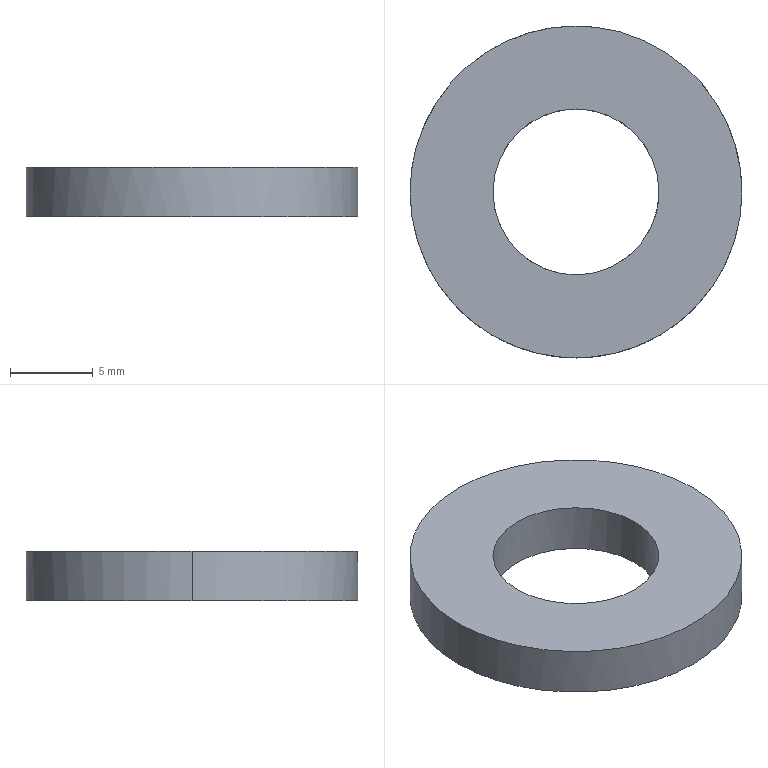Part | STEP file | Positioning_id2190_x_t | 1 solid | 6 faces | box 20 x 20 x 3 mm | volume 706.858 mm3 | cylinder 4 | plane 2 | commonest cylinder face diameters 10 x2 20 x2
STEP:
#1=CARTESIAN_POINT('',(0.,0.,0.));
#2=DIRECTION('',(0.,0.,1.));
#3=DIRECTION('',(1.,0.,0.));
#4=AXIS2_PLACEMENT_3D('',#1,#2,#3);
#5=CARTESIAN_POINT('',(-1002.502,421.,51.5));
#6=VERTEX_POINT('',#5);
#7=CARTESIAN_POINT('',(-1007.502,416.,51.5));
#8=VERTEX_POINT('',#7);
#9=CARTESIAN_POINT('',(-1002.502,416.,51.5));
#10=DIRECTION('',(0.,0.,1.));
#11=DIRECTION('',(0.,1.,0.));
#12=AXIS2_PLACEMENT_3D('',#9,#10,#11);
#13=CIRCLE('',#12,5.);
#14=CARTESIAN_POINT('',(-1002.502,416.,48.5));
#15=DIRECTION('',(0.,0.,-1.));
#16=DIRECTION('',(-1.,0.,0.));
#17=AXIS2_PLACEMENT_3D('',#14,#15,#16);
#18=CYLINDRICAL_SURFACE('',#17,5.);
#19=CARTESIAN_POINT('',(1.571,-3.));
#20=DIRECTION('',(-1.,0.));
#21=VECTOR('',#20,1.);
#22=LINE('',#19,#21);
#23=(GEOMETRIC_REPRESENTATION_CONTEXT(2)PARAMETRIC_REPRESENTATION_CONTEXT()REPRESENTATION_CONTEXT('',''));
#24=DEFINITIONAL_REPRESENTATION('',(#22),#23);
#25=PCURVE('',#18,#24);
#26=CARTESIAN_POINT('',(-1002.502,416.,51.5));
#27=DIRECTION('',(0.,0.,1.));
#28=DIRECTION('',(-1.,0.,0.));
#29=AXIS2_PLACEMENT_3D('',#26,#27,#28);
#30=PLANE('',#29);
#31=CARTESIAN_POINT('',(0.,0.));
#32=DIRECTION('',(0.,-1.));
#33=AXIS2_PLACEMENT_2D('',#31,#32);
#34=CIRCLE('',#33,5.);
#35=(GEOMETRIC_REPRESENTATION_CONTEXT(2)PARAMETRIC_REPRESENTATION_CONTEXT()REPRESENTATION_CONTEXT('',''));
#36=DEFINITIONAL_REPRESENTATION('',(#34),#35);
#37=PCURVE('',#30,#36);
#38=SURFACE_CURVE('',#13,(#25,#37),.PCURVE_S1.);
#39=EDGE_CURVE('',#6,#8,#38,.T.);
#40=ORIENTED_EDGE('',*,*,#39,.F.);
#41=CARTESIAN_POINT('',(-997.502,416.,51.5));
#42=VERTEX_POINT('',#41);
#43=CARTESIAN_POINT('',(-1002.502,416.,51.5));
#44=DIRECTION('',(0.,0.,1.));
#45=DIRECTION('',(0.,1.,0.));
#46=AXIS2_PLACEMENT_3D('',#43,#44,#45);
#47=CIRCLE('',#46,5.);
#48=CARTESIAN_POINT('',(7.854,-3.));
#49=DIRECTION('',(-1.,0.));
#50=VECTOR('',#49,1.);
#51=LINE('',#48,#50);
#52=(GEOMETRIC_REPRESENTATION_CONTEXT(2)PARAMETRIC_REPRESENTATION_CONTEXT()REPRESENTATION_CONTEXT('',''));
#53=DEFINITIONAL_REPRESENTATION('',(#51),#52);
#54=PCURVE('',#18,#53);
#55=CARTESIAN_POINT('',(0.,0.));
#56=DIRECTION('',(0.,-1.));
#57=AXIS2_PLACEMENT_2D('',#55,#56);
#58=CIRCLE('',#57,5.);
#59=(GEOMETRIC_REPRESENTATION_CONTEXT(2)PARAMETRIC_REPRESENTATION_CONTEXT()REPRESENTATION_CONTEXT('',''));
#60=DEFINITIONAL_REPRESENTATION('',(#58),#59);
#61=PCURVE('',#30,#60);
#62=SURFACE_CURVE('',#47,(#54,#61),.PCURVE_S1.);
#63=EDGE_CURVE('',#42,#6,#62,.T.);
#64=ORIENTED_EDGE('',*,*,#63,.F.);
#65=CARTESIAN_POINT('',(-997.502,416.,48.5));
#66=VERTEX_POINT('',#65);
#67=CARTESIAN_POINT('',(-997.502,416.,48.5));
#68=DIRECTION('',(0.,0.,1.));
#69=VECTOR('',#68,1.);
#70=LINE('',#67,#69);
#71=CARTESIAN_POINT('',(3.142,0.));
#72=DIRECTION('',(0.,-1.));
#73=VECTOR('',#72,1.);
#74=LINE('',#71,#73);
#75=(GEOMETRIC_REPRESENTATION_CONTEXT(2)PARAMETRIC_REPRESENTATION_CONTEXT()REPRESENTATION_CONTEXT('',''));
#76=DEFINITIONAL_REPRESENTATION('',(#74),#75);
#77=PCURVE('',#18,#76);
#78=CARTESIAN_POINT('',(-1002.502,416.,48.5));
#79=DIRECTION('',(0.,0.,-1.));
#80=DIRECTION('',(-1.,0.,0.));
#81=AXIS2_PLACEMENT_3D('',#78,#79,#80);
#82=CYLINDRICAL_SURFACE('',#81,5.);
#83=CARTESIAN_POINT('',(3.142,0.));
#84=DIRECTION('',(0.,-1.));
#85=VECTOR('',#84,1.);
#86=LINE('',#83,#85);
#87=(GEOMETRIC_REPRESENTATION_CONTEXT(2)PARAMETRIC_REPRESENTATION_CONTEXT()REPRESENTATION_CONTEXT('',''));
#88=DEFINITIONAL_REPRESENTATION('',(#86),#87);
#89=PCURVE('',#82,#88);
#90=SURFACE_CURVE('',#70,(#77,#89),.PCURVE_S1.);
#91=EDGE_CURVE('',#66,#42,#90,.T.);
#92=ORIENTED_EDGE('',*,*,#91,.F.);
#93=CARTESIAN_POINT('',(-1007.502,416.,48.5));
#94=VERTEX_POINT('',#93);
#95=CARTESIAN_POINT('',(-1002.502,416.,48.5));
#96=DIRECTION('',(0.,0.,-1.));
#97=DIRECTION('',(0.,1.,0.));
#98=AXIS2_PLACEMENT_3D('',#95,#96,#97);
#99=CIRCLE('',#98,5.);
#100=CARTESIAN_POINT('',(-4.712,0.));
#101=DIRECTION('',(1.,0.));
#102=VECTOR('',#101,1.);
#103=LINE('',#100,#102);
#104=(GEOMETRIC_REPRESENTATION_CONTEXT(2)PARAMETRIC_REPRESENTATION_CONTEXT()REPRESENTATION_CONTEXT('',''));
#105=DEFINITIONAL_REPRESENTATION('',(#103),#104);
#106=PCURVE('',#18,#105);
#107=CARTESIAN_POINT('',(-1002.502,416.,48.5));
#108=DIRECTION('',(0.,0.,-1.));
#109=DIRECTION('',(1.,0.,0.));
#110=AXIS2_PLACEMENT_3D('',#107,#108,#109);
#111=PLANE('',#110);
#112=CARTESIAN_POINT('',(0.,0.));
#113=DIRECTION('',(0.,-1.));
#114=AXIS2_PLACEMENT_2D('',#112,#113);
#115=CIRCLE('',#114,5.);
#116=(GEOMETRIC_REPRESENTATION_CONTEXT(2)PARAMETRIC_REPRESENTATION_CONTEXT()REPRESENTATION_CONTEXT('',''));
#117=DEFINITIONAL_REPRESENTATION('',(#115),#116);
#118=PCURVE('',#111,#117);
#119=SURFACE_CURVE('',#99,(#106,#118),.PCURVE_S1.);
#120=EDGE_CURVE('',#94,#66,#119,.T.);
#121=ORIENTED_EDGE('',*,*,#120,.F.);
#122=CARTESIAN_POINT('',(-1007.502,416.,48.5));
#123=DIRECTION('',(0.,0.,-1.));
#124=VECTOR('',#123,1.);
#125=LINE('',#122,#124);
#126=CARTESIAN_POINT('',(0.,0.));
#127=DIRECTION('',(0.,1.));
#128=VECTOR('',#127,1.);
#129=LINE('',#126,#128);
#130=(GEOMETRIC_REPRESENTATION_CONTEXT(2)PARAMETRIC_REPRESENTATION_CONTEXT()REPRESENTATION_CONTEXT('',''));
#131=DEFINITIONAL_REPRESENTATION('',(#129),#130);
#132=PCURVE('',#18,#131);
#133=CARTESIAN_POINT('',(6.283,0.));
#134=DIRECTION('',(0.,1.));
#135=VECTOR('',#134,1.);
#136=LINE('',#133,#135);
#137=(GEOMETRIC_REPRESENTATION_CONTEXT(2)PARAMETRIC_REPRESENTATION_CONTEXT()REPRESENTATION_CONTEXT('',''));
#138=DEFINITIONAL_REPRESENTATION('',(#136),#137);
#139=PCURVE('',#82,#138);
#140=SURFACE_CURVE('',#125,(#132,#139),.PCURVE_S1.);
#141=EDGE_CURVE('',#8,#94,#140,.T.);
#142=ORIENTED_EDGE('',*,*,#141,.F.);
#143=EDGE_LOOP('',(#40,#64,#92,#121,#142));
#144=FACE_BOUND('',#143,.F.);
#145=ADVANCED_FACE('',(#144),#18,.F.);
#146=CARTESIAN_POINT('',(-1012.502,416.,51.5));
#147=VERTEX_POINT('',#146);
#148=CARTESIAN_POINT('',(-1012.502,416.,48.5));
#149=VERTEX_POINT('',#148);
#150=CARTESIAN_POINT('',(-1012.502,416.,48.5));
#151=DIRECTION('',(0.,0.,-1.));
#152=VECTOR('',#151,1.);
#153=LINE('',#150,#152);
#154=CARTESIAN_POINT('',(-1002.502,416.,48.5));
#155=DIRECTION('',(0.,0.,-1.));
#156=DIRECTION('',(-1.,0.,0.));
#157=AXIS2_PLACEMENT_3D('',#154,#155,#156);
#158=CYLINDRICAL_SURFACE('',#157,10.);
#159=CARTESIAN_POINT('',(6.283,0.));
#160=DIRECTION('',(0.,1.));
#161=VECTOR('',#160,1.);
#162=LINE('',#159,#161);
#163=(GEOMETRIC_REPRESENTATION_CONTEXT(2)PARAMETRIC_REPRESENTATION_CONTEXT()REPRESENTATION_CONTEXT('',''));
#164=DEFINITIONAL_REPRESENTATION('',(#162),#163);
#165=PCURVE('',#158,#164);
#166=CARTESIAN_POINT('',(-1002.502,416.,48.5));
#167=DIRECTION('',(0.,0.,-1.));
#168=DIRECTION('',(-1.,0.,0.));
#169=AXIS2_PLACEMENT_3D('',#166,#167,#168);
#170=CYLINDRICAL_SURFACE('',#169,10.);
#171=CARTESIAN_POINT('',(0.,0.));
#172=DIRECTION('',(0.,1.));
#173=VECTOR('',#172,1.);
#174=LINE('',#171,#173);
#175=(GEOMETRIC_REPRESENTATION_CONTEXT(2)PARAMETRIC_REPRESENTATION_CONTEXT()REPRESENTATION_CONTEXT('',''));
#176=DEFINITIONAL_REPRESENTATION('',(#174),#175);
#177=PCURVE('',#170,#176);
#178=SURFACE_CURVE('',#153,(#165,#177),.PCURVE_S1.);
#179=EDGE_CURVE('',#147,#149,#178,.T.);
#180=ORIENTED_EDGE('',*,*,#179,.T.);
#181=CARTESIAN_POINT('',(-1002.502,406.,48.5));
#182=VERTEX_POINT('',#181);
#183=CARTESIAN_POINT('',(-1002.502,416.,48.5));
#184=DIRECTION('',(0.,0.,-1.));
#185=DIRECTION('',(0.,1.,0.));
#186=AXIS2_PLACEMENT_3D('',#183,#184,#185);
#187=CIRCLE('',#186,10.);
#188=CARTESIAN_POINT('',(1.571,0.));
#189=DIRECTION('',(1.,0.));
#190=VECTOR('',#189,1.);
#191=LINE('',#188,#190);
#192=(GEOMETRIC_REPRESENTATION_CONTEXT(2)PARAMETRIC_REPRESENTATION_CONTEXT()REPRESENTATION_CONTEXT('',''));
#193=DEFINITIONAL_REPRESENTATION('',(#191),#192);
#194=PCURVE('',#158,#193);
#195=CARTESIAN_POINT('',(0.,0.));
#196=DIRECTION('',(0.,-1.));
#197=AXIS2_PLACEMENT_2D('',#195,#196);
#198=CIRCLE('',#197,10.);
#199=(GEOMETRIC_REPRESENTATION_CONTEXT(2)PARAMETRIC_REPRESENTATION_CONTEXT()REPRESENTATION_CONTEXT('',''));
#200=DEFINITIONAL_REPRESENTATION('',(#198),#199);
#201=PCURVE('',#111,#200);
#202=SURFACE_CURVE('',#187,(#194,#201),.PCURVE_S1.);
#203=EDGE_CURVE('',#182,#149,#202,.T.);
#204=ORIENTED_EDGE('',*,*,#203,.F.);
#205=CARTESIAN_POINT('',(-992.502,416.,48.5));
#206=VERTEX_POINT('',#205);
#207=CARTESIAN_POINT('',(-1002.502,416.,48.5));
#208=DIRECTION('',(0.,0.,-1.));
#209=DIRECTION('',(0.,1.,0.));
#210=AXIS2_PLACEMENT_3D('',#207,#208,#209);
#211=CIRCLE('',#210,10.);
#212=CARTESIAN_POINT('',(1.571,0.));
#213=DIRECTION('',(1.,0.));
#214=VECTOR('',#213,1.);
#215=LINE('',#212,#214);
#216=(GEOMETRIC_REPRESENTATION_CONTEXT(2)PARAMETRIC_REPRESENTATION_CONTEXT()REPRESENTATION_CONTEXT('',''));
#217=DEFINITIONAL_REPRESENTATION('',(#215),#216);
#218=PCURVE('',#158,#217);
#219=CARTESIAN_POINT('',(0.,0.));
#220=DIRECTION('',(0.,-1.));
#221=AXIS2_PLACEMENT_2D('',#219,#220);
#222=CIRCLE('',#221,10.);
#223=(GEOMETRIC_REPRESENTATION_CONTEXT(2)PARAMETRIC_REPRESENTATION_CONTEXT()REPRESENTATION_CONTEXT('',''));
#224=DEFINITIONAL_REPRESENTATION('',(#222),#223);
#225=PCURVE('',#111,#224);
#226=SURFACE_CURVE('',#211,(#218,#225),.PCURVE_S1.);
#227=EDGE_CURVE('',#206,#182,#226,.T.);
#228=ORIENTED_EDGE('',*,*,#227,.F.);
#229=CARTESIAN_POINT('',(-992.502,416.,51.5));
#230=VERTEX_POINT('',#229);
#231=CARTESIAN_POINT('',(-992.502,416.,48.5));
#232=DIRECTION('',(0.,0.,1.));
#233=VECTOR('',#232,1.);
#234=LINE('',#231,#233);
#235=CARTESIAN_POINT('',(3.142,0.));
#236=DIRECTION('',(0.,-1.));
#237=VECTOR('',#236,1.);
#238=LINE('',#235,#237);
#239=(GEOMETRIC_REPRESENTATION_CONTEXT(2)PARAMETRIC_REPRESENTATION_CONTEXT()REPRESENTATION_CONTEXT('',''));
#240=DEFINITIONAL_REPRESENTATION('',(#238),#239);
#241=PCURVE('',#158,#240);
#242=CARTESIAN_POINT('',(3.142,0.));
#243=DIRECTION('',(0.,-1.));
#244=VECTOR('',#243,1.);
#245=LINE('',#242,#244);
#246=(GEOMETRIC_REPRESENTATION_CONTEXT(2)PARAMETRIC_REPRESENTATION_CONTEXT()REPRESENTATION_CONTEXT('',''));
#247=DEFINITIONAL_REPRESENTATION('',(#245),#246);
#248=PCURVE('',#170,#247);
#249=SURFACE_CURVE('',#234,(#241,#248),.PCURVE_S1.);
#250=EDGE_CURVE('',#206,#230,#249,.T.);
#251=ORIENTED_EDGE('',*,*,#250,.T.);
#252=CARTESIAN_POINT('',(-1002.502,416.,51.5));
#253=DIRECTION('',(0.,0.,1.));
#254=DIRECTION('',(0.,1.,0.));
#255=AXIS2_PLACEMENT_3D('',#252,#253,#254);
#256=CIRCLE('',#255,10.);
#257=CARTESIAN_POINT('',(7.854,-3.));
#258=DIRECTION('',(-1.,0.));
#259=VECTOR('',#258,1.);
#260=LINE('',#257,#259);
#261=(GEOMETRIC_REPRESENTATION_CONTEXT(2)PARAMETRIC_REPRESENTATION_CONTEXT()REPRESENTATION_CONTEXT('',''));
#262=DEFINITIONAL_REPRESENTATION('',(#260),#261);
#263=PCURVE('',#158,#262);
#264=CARTESIAN_POINT('',(0.,0.));
#265=DIRECTION('',(0.,-1.));
#266=AXIS2_PLACEMENT_2D('',#264,#265);
#267=CIRCLE('',#266,10.);
#268=(GEOMETRIC_REPRESENTATION_CONTEXT(2)PARAMETRIC_REPRESENTATION_CONTEXT()REPRESENTATION_CONTEXT('',''));
#269=DEFINITIONAL_REPRESENTATION('',(#267),#268);
#270=PCURVE('',#30,#269);
#271=SURFACE_CURVE('',#256,(#263,#270),.PCURVE_S1.);
#272=EDGE_CURVE('',#147,#230,#271,.T.);
#273=ORIENTED_EDGE('',*,*,#272,.F.);
#274=EDGE_LOOP('',(#180,#204,#228,#251,#273));
#275=FACE_BOUND('',#274,.T.);
#276=ADVANCED_FACE('',(#275),#158,.T.);
#277=CARTESIAN_POINT('',(-1002.502,411.,48.5));
#278=VERTEX_POINT('',#277);
#279=CARTESIAN_POINT('',(-997.502,416.,48.5));
#280=CARTESIAN_POINT('',(-997.502,411.,48.5));
#281=CARTESIAN_POINT('',(-1002.502,411.,48.5));
#282=(BOUNDED_CURVE()B_SPLINE_CURVE(2,(#279,#280,#281),.UNSPECIFIED.,.F.,.F.)B_SPLINE_CURVE_WITH_KNOTS((3,3),(0.,1.),.PIECEWISE_BEZIER_KNOTS.)CURVE()GEOMETRIC_REPRESENTATION_ITEM()RATIONAL_B_SPLINE_CURVE((1.,0.7071,1.))REPRESENTATION_ITEM(''));
#283=CARTESIAN_POINT('',(5.,0.));
#284=CARTESIAN_POINT('',(5.,5.));
#285=CARTESIAN_POINT('',(0.,5.));
#286=(BOUNDED_CURVE()B_SPLINE_CURVE(2,(#283,#284,#285),.UNSPECIFIED.,.F.,.F.)B_SPLINE_CURVE_WITH_KNOTS((3,3),(0.,1.),.PIECEWISE_BEZIER_KNOTS.)CURVE()GEOMETRIC_REPRESENTATION_ITEM()RATIONAL_B_SPLINE_CURVE((1.,0.7071,1.))REPRESENTATION_ITEM(''));
#287=(GEOMETRIC_REPRESENTATION_CONTEXT(2)PARAMETRIC_REPRESENTATION_CONTEXT()REPRESENTATION_CONTEXT('',''));
#288=DEFINITIONAL_REPRESENTATION('',(#286),#287);
#289=PCURVE('',#111,#288);
#290=CARTESIAN_POINT('',(3.142,0.));
#291=CARTESIAN_POINT('',(3.163,0.));
#292=CARTESIAN_POINT('',(3.206,0.));
#293=CARTESIAN_POINT('',(3.273,0.));
#294=CARTESIAN_POINT('',(3.342,0.));
#295=CARTESIAN_POINT('',(3.411,0.));
#296=CARTESIAN_POINT('',(3.482,0.));
#297=CARTESIAN_POINT('',(3.555,0.));
#298=CARTESIAN_POINT('',(3.628,0.));
#299=CARTESIAN_POINT('',(3.702,0.));
#300=CARTESIAN_POINT('',(3.777,0.));
#301=CARTESIAN_POINT('',(3.852,0.));
#302=CARTESIAN_POINT('',(3.927,0.));
#303=CARTESIAN_POINT('',(4.002,0.));
#304=CARTESIAN_POINT('',(4.077,0.));
#305=CARTESIAN_POINT('',(4.152,0.));
#306=CARTESIAN_POINT('',(4.226,0.));
#307=CARTESIAN_POINT('',(4.299,0.));
#308=CARTESIAN_POINT('',(4.372,0.));
#309=CARTESIAN_POINT('',(4.443,0.));
#310=CARTESIAN_POINT('',(4.512,0.));
#311=CARTESIAN_POINT('',(4.581,0.));
#312=CARTESIAN_POINT('',(4.648,0.));
#313=CARTESIAN_POINT('',(4.691,0.));
#314=CARTESIAN_POINT('',(4.712,0.));
#315=B_SPLINE_CURVE_WITH_KNOTS('',3,(#290,#291,#292,#293,#294,#295,#296,#297,#298,#299,#300,#301,#302,#303,#304,#305,#306,#307,#308,#309,#310,#311,#312,#313,#314),.UNSPECIFIED.,.F.,.F.,(4,1,1,1,1,1,1,1,1,1,1,1,1,1,1,1,1,1,1,1,1,1,4),(0.,0.04545,0.09091,0.1364,0.1818,0.2273,0.2727,0.3182,0.3636,0.4091,0.4545,0.5,0.5455,0.5909,0.6364,0.6818,0.7273,0.7727,0.8182,0.8636,0.9091,0.9545,1.),.QUASI_UNIFORM_KNOTS.);
#316=(GEOMETRIC_REPRESENTATION_CONTEXT(2)PARAMETRIC_REPRESENTATION_CONTEXT()REPRESENTATION_CONTEXT('',''));
#317=DEFINITIONAL_REPRESENTATION('',(#315),#316);
#318=PCURVE('',#82,#317);
#319=SURFACE_CURVE('',#282,(#289,#318),.PCURVE_S1.);
#320=EDGE_CURVE('',#66,#278,#319,.T.);
#321=ORIENTED_EDGE('',*,*,#320,.F.);
#322=ORIENTED_EDGE('',*,*,#120,.F.);
#323=CARTESIAN_POINT('',(-1002.502,411.,48.5));
#324=CARTESIAN_POINT('',(-1007.502,411.,48.5));
#325=CARTESIAN_POINT('',(-1007.502,416.,48.5));
#326=(BOUNDED_CURVE()B_SPLINE_CURVE(2,(#323,#324,#325),.UNSPECIFIED.,.F.,.F.)B_SPLINE_CURVE_WITH_KNOTS((3,3),(0.,1.),.PIECEWISE_BEZIER_KNOTS.)CURVE()GEOMETRIC_REPRESENTATION_ITEM()RATIONAL_B_SPLINE_CURVE((1.,0.7071,1.))REPRESENTATION_ITEM(''));
#327=CARTESIAN_POINT('',(0.,5.));
#328=CARTESIAN_POINT('',(-5.,5.));
#329=CARTESIAN_POINT('',(-5.,0.));
#330=(BOUNDED_CURVE()B_SPLINE_CURVE(2,(#327,#328,#329),.UNSPECIFIED.,.F.,.F.)B_SPLINE_CURVE_WITH_KNOTS((3,3),(0.,1.),.PIECEWISE_BEZIER_KNOTS.)CURVE()GEOMETRIC_REPRESENTATION_ITEM()RATIONAL_B_SPLINE_CURVE((1.,0.7071,1.))REPRESENTATION_ITEM(''));
#331=(GEOMETRIC_REPRESENTATION_CONTEXT(2)PARAMETRIC_REPRESENTATION_CONTEXT()REPRESENTATION_CONTEXT('',''));
#332=DEFINITIONAL_REPRESENTATION('',(#330),#331);
#333=PCURVE('',#111,#332);
#334=CARTESIAN_POINT('',(4.712,0.));
#335=CARTESIAN_POINT('',(4.734,0.));
#336=CARTESIAN_POINT('',(4.777,0.));
#337=CARTESIAN_POINT('',(4.844,0.));
#338=CARTESIAN_POINT('',(4.912,0.));
#339=CARTESIAN_POINT('',(4.982,0.));
#340=CARTESIAN_POINT('',(5.053,0.));
#341=CARTESIAN_POINT('',(5.125,0.));
#342=CARTESIAN_POINT('',(5.199,0.));
#343=CARTESIAN_POINT('',(5.273,0.));
#344=CARTESIAN_POINT('',(5.347,0.));
#345=CARTESIAN_POINT('',(5.422,0.));
#346=CARTESIAN_POINT('',(5.498,0.));
#347=CARTESIAN_POINT('',(5.573,0.));
#348=CARTESIAN_POINT('',(5.648,0.));
#349=CARTESIAN_POINT('',(5.723,0.));
#350=CARTESIAN_POINT('',(5.797,0.));
#351=CARTESIAN_POINT('',(5.87,0.));
#352=CARTESIAN_POINT('',(5.942,0.));
#353=CARTESIAN_POINT('',(6.013,0.));
#354=CARTESIAN_POINT('',(6.083,0.));
#355=CARTESIAN_POINT('',(6.152,0.));
#356=CARTESIAN_POINT('',(6.218,0.));
#357=CARTESIAN_POINT('',(6.262,0.));
#358=CARTESIAN_POINT('',(6.283,0.));
#359=B_SPLINE_CURVE_WITH_KNOTS('',3,(#334,#335,#336,#337,#338,#339,#340,#341,#342,#343,#344,#345,#346,#347,#348,#349,#350,#351,#352,#353,#354,#355,#356,#357,#358),.UNSPECIFIED.,.F.,.F.,(4,1,1,1,1,1,1,1,1,1,1,1,1,1,1,1,1,1,1,1,1,1,4),(0.,0.04545,0.09091,0.1364,0.1818,0.2273,0.2727,0.3182,0.3636,0.4091,0.4545,0.5,0.5455,0.5909,0.6364,0.6818,0.7273,0.7727,0.8182,0.8636,0.9091,0.9545,1.),.QUASI_UNIFORM_KNOTS.);
#360=(GEOMETRIC_REPRESENTATION_CONTEXT(2)PARAMETRIC_REPRESENTATION_CONTEXT()REPRESENTATION_CONTEXT('',''));
#361=DEFINITIONAL_REPRESENTATION('',(#359),#360);
#362=PCURVE('',#82,#361);
#363=SURFACE_CURVE('',#326,(#333,#362),.PCURVE_S1.);
#364=EDGE_CURVE('',#278,#94,#363,.T.);
#365=ORIENTED_EDGE('',*,*,#364,.F.);
#366=EDGE_LOOP('',(#321,#322,#365));
#367=FACE_BOUND('',#366,.T.);
#368=ORIENTED_EDGE('',*,*,#227,.T.);
#369=ORIENTED_EDGE('',*,*,#203,.T.);
#370=CARTESIAN_POINT('',(-1012.502,416.,48.5));
#371=CARTESIAN_POINT('',(-1012.502,426.,48.5));
#372=CARTESIAN_POINT('',(-1002.502,431.,48.5));
#373=CARTESIAN_POINT('',(-992.502,426.,48.5));
#374=CARTESIAN_POINT('',(-992.502,416.,48.5));
#375=(BOUNDED_CURVE()B_SPLINE_CURVE(4,(#370,#371,#372,#373,#374),.UNSPECIFIED.,.F.,.F.)B_SPLINE_CURVE_WITH_KNOTS((5,5),(0.,1.),.PIECEWISE_BEZIER_KNOTS.)CURVE()GEOMETRIC_REPRESENTATION_ITEM()RATIONAL_B_SPLINE_CURVE((1.,0.7071,0.6667,0.7071,1.))REPRESENTATION_ITEM(''));
#376=CARTESIAN_POINT('',(-10.,0.));
#377=CARTESIAN_POINT('',(-10.,-10.));
#378=CARTESIAN_POINT('',(0.,-15.));
#379=CARTESIAN_POINT('',(10.,-10.));
#380=CARTESIAN_POINT('',(10.,0.));
#381=(BOUNDED_CURVE()B_SPLINE_CURVE(4,(#376,#377,#378,#379,#380),.UNSPECIFIED.,.F.,.F.)B_SPLINE_CURVE_WITH_KNOTS((5,5),(0.,1.),.PIECEWISE_BEZIER_KNOTS.)CURVE()GEOMETRIC_REPRESENTATION_ITEM()RATIONAL_B_SPLINE_CURVE((1.,0.7071,0.6667,0.7071,1.))REPRESENTATION_ITEM(''));
#382=(GEOMETRIC_REPRESENTATION_CONTEXT(2)PARAMETRIC_REPRESENTATION_CONTEXT()REPRESENTATION_CONTEXT('',''));
#383=DEFINITIONAL_REPRESENTATION('',(#381),#382);
#384=PCURVE('',#111,#383);
#385=CARTESIAN_POINT('',(0.,0.));
#386=CARTESIAN_POINT('',(0.04285,0.));
#387=CARTESIAN_POINT('',(0.1297,0.));
#388=CARTESIAN_POINT('',(0.2633,0.));
#389=CARTESIAN_POINT('',(0.3999,0.));
#390=CARTESIAN_POINT('',(0.5394,0.));
#391=CARTESIAN_POINT('',(0.6816,0.));
#392=CARTESIAN_POINT('',(0.8261,0.));
#393=CARTESIAN_POINT('',(0.9725,0.));
#394=CARTESIAN_POINT('',(1.121,0.));
#395=CARTESIAN_POINT('',(1.27,0.));
#396=CARTESIAN_POINT('',(1.42,0.));
#397=CARTESIAN_POINT('',(1.571,0.));
#398=CARTESIAN_POINT('',(1.721,0.));
#399=CARTESIAN_POINT('',(1.872,0.));
#400=CARTESIAN_POINT('',(2.021,0.));
#401=CARTESIAN_POINT('',(2.169,0.));
#402=CARTESIAN_POINT('',(2.316,0.));
#403=CARTESIAN_POINT('',(2.46,0.));
#404=CARTESIAN_POINT('',(2.602,0.));
#405=CARTESIAN_POINT('',(2.742,0.));
#406=CARTESIAN_POINT('',(2.878,0.));
#407=CARTESIAN_POINT('',(3.012,0.));
#408=CARTESIAN_POINT('',(3.099,0.));
#409=CARTESIAN_POINT('',(3.142,0.));
#410=B_SPLINE_CURVE_WITH_KNOTS('',3,(#385,#386,#387,#388,#389,#390,#391,#392,#393,#394,#395,#396,#397,#398,#399,#400,#401,#402,#403,#404,#405,#406,#407,#408,#409),.UNSPECIFIED.,.F.,.F.,(4,1,1,1,1,1,1,1,1,1,1,1,1,1,1,1,1,1,1,1,1,1,4),(0.,0.04545,0.09091,0.1364,0.1818,0.2273,0.2727,0.3182,0.3636,0.4091,0.4545,0.5,0.5455,0.5909,0.6364,0.6818,0.7273,0.7727,0.8182,0.8636,0.9091,0.9545,1.),.QUASI_UNIFORM_KNOTS.);
#411=(GEOMETRIC_REPRESENTATION_CONTEXT(2)PARAMETRIC_REPRESENTATION_CONTEXT()REPRESENTATION_CONTEXT('',''));
#412=DEFINITIONAL_REPRESENTATION('',(#410),#411);
#413=PCURVE('',#170,#412);
#414=SURFACE_CURVE('',#375,(#384,#413),.PCURVE_S1.);
#415=EDGE_CURVE('',#149,#206,#414,.T.);
#416=ORIENTED_EDGE('',*,*,#415,.T.);
#417=EDGE_LOOP('',(#368,#369,#416));
#418=FACE_BOUND('',#417,.T.);
#419=ADVANCED_FACE('',(#367,#418),#111,.T.);
#420=ORIENTED_EDGE('',*,*,#63,.F.);
#421=CARTESIAN_POINT('',(-1007.502,416.,51.5));
#422=CARTESIAN_POINT('',(-1007.502,411.,51.5));
#423=CARTESIAN_POINT('',(-1002.502,408.5,51.5));
#424=CARTESIAN_POINT('',(-997.502,411.,51.5));
#425=CARTESIAN_POINT('',(-997.502,416.,51.5));
#426=(BOUNDED_CURVE()B_SPLINE_CURVE(4,(#421,#422,#423,#424,#425),.UNSPECIFIED.,.F.,.F.)B_SPLINE_CURVE_WITH_KNOTS((5,5),(0.,1.),.PIECEWISE_BEZIER_KNOTS.)CURVE()GEOMETRIC_REPRESENTATION_ITEM()RATIONAL_B_SPLINE_CURVE((1.,0.7071,0.6667,0.7071,1.))REPRESENTATION_ITEM(''));
#427=CARTESIAN_POINT('',(5.,0.));
#428=CARTESIAN_POINT('',(5.,5.));
#429=CARTESIAN_POINT('',(0.,7.5));
#430=CARTESIAN_POINT('',(-5.,5.));
#431=CARTESIAN_POINT('',(-5.,0.));
#432=(BOUNDED_CURVE()B_SPLINE_CURVE(4,(#427,#428,#429,#430,#431),.UNSPECIFIED.,.F.,.F.)B_SPLINE_CURVE_WITH_KNOTS((5,5),(0.,1.),.PIECEWISE_BEZIER_KNOTS.)CURVE()GEOMETRIC_REPRESENTATION_ITEM()RATIONAL_B_SPLINE_CURVE((1.,0.7071,0.6667,0.7071,1.))REPRESENTATION_ITEM(''));
#433=(GEOMETRIC_REPRESENTATION_CONTEXT(2)PARAMETRIC_REPRESENTATION_CONTEXT()REPRESENTATION_CONTEXT('',''));
#434=DEFINITIONAL_REPRESENTATION('',(#432),#433);
#435=PCURVE('',#30,#434);
#436=CARTESIAN_POINT('',(6.283,-3.));
#437=CARTESIAN_POINT('',(6.24,-3.));
#438=CARTESIAN_POINT('',(6.153,-3.));
#439=CARTESIAN_POINT('',(6.02,-3.));
#440=CARTESIAN_POINT('',(5.883,-3.));
#441=CARTESIAN_POINT('',(5.744,-3.));
#442=CARTESIAN_POINT('',(5.602,-3.));
#443=CARTESIAN_POINT('',(5.457,-3.));
#444=CARTESIAN_POINT('',(5.311,-3.));
#445=CARTESIAN_POINT('',(5.163,-3.));
#446=CARTESIAN_POINT('',(5.013,-3.));
#447=CARTESIAN_POINT('',(4.863,-3.));
#448=CARTESIAN_POINT('',(4.712,-3.));
#449=CARTESIAN_POINT('',(4.562,-3.));
#450=CARTESIAN_POINT('',(4.412,-3.));
#451=CARTESIAN_POINT('',(4.262,-3.));
#452=CARTESIAN_POINT('',(4.114,-3.));
#453=CARTESIAN_POINT('',(3.968,-3.));
#454=CARTESIAN_POINT('',(3.823,-3.));
#455=CARTESIAN_POINT('',(3.681,-3.));
#456=CARTESIAN_POINT('',(3.542,-3.));
#457=CARTESIAN_POINT('',(3.405,-3.));
#458=CARTESIAN_POINT('',(3.271,-3.));
#459=CARTESIAN_POINT('',(3.184,-3.));
#460=CARTESIAN_POINT('',(3.142,-3.));
#461=B_SPLINE_CURVE_WITH_KNOTS('',3,(#436,#437,#438,#439,#440,#441,#442,#443,#444,#445,#446,#447,#448,#449,#450,#451,#452,#453,#454,#455,#456,#457,#458,#459,#460),.UNSPECIFIED.,.F.,.F.,(4,1,1,1,1,1,1,1,1,1,1,1,1,1,1,1,1,1,1,1,1,1,4),(0.,0.04545,0.09091,0.1364,0.1818,0.2273,0.2727,0.3182,0.3636,0.4091,0.4545,0.5,0.5455,0.5909,0.6364,0.6818,0.7273,0.7727,0.8182,0.8636,0.9091,0.9545,1.),.QUASI_UNIFORM_KNOTS.);
#462=(GEOMETRIC_REPRESENTATION_CONTEXT(2)PARAMETRIC_REPRESENTATION_CONTEXT()REPRESENTATION_CONTEXT('',''));
#463=DEFINITIONAL_REPRESENTATION('',(#461),#462);
#464=PCURVE('',#82,#463);
#465=SURFACE_CURVE('',#426,(#435,#464),.PCURVE_S1.);
#466=EDGE_CURVE('',#8,#42,#465,.T.);
#467=ORIENTED_EDGE('',*,*,#466,.F.);
#468=ORIENTED_EDGE('',*,*,#39,.F.);
#469=EDGE_LOOP('',(#420,#467,#468));
#470=FACE_BOUND('',#469,.T.);
#471=CARTESIAN_POINT('',(-1002.502,426.,51.5));
#472=VERTEX_POINT('',#471);
#473=CARTESIAN_POINT('',(-992.502,416.,51.5));
#474=CARTESIAN_POINT('',(-992.502,426.,51.5));
#475=CARTESIAN_POINT('',(-1002.502,426.,51.5));
#476=(BOUNDED_CURVE()B_SPLINE_CURVE(2,(#473,#474,#475),.UNSPECIFIED.,.F.,.F.)B_SPLINE_CURVE_WITH_KNOTS((3,3),(0.,1.),.PIECEWISE_BEZIER_KNOTS.)CURVE()GEOMETRIC_REPRESENTATION_ITEM()RATIONAL_B_SPLINE_CURVE((1.,0.7071,1.))REPRESENTATION_ITEM(''));
#477=CARTESIAN_POINT('',(-10.,0.));
#478=CARTESIAN_POINT('',(-10.,-10.));
#479=CARTESIAN_POINT('',(0.,-10.));
#480=(BOUNDED_CURVE()B_SPLINE_CURVE(2,(#477,#478,#479),.UNSPECIFIED.,.F.,.F.)B_SPLINE_CURVE_WITH_KNOTS((3,3),(0.,1.),.PIECEWISE_BEZIER_KNOTS.)CURVE()GEOMETRIC_REPRESENTATION_ITEM()RATIONAL_B_SPLINE_CURVE((1.,0.7071,1.))REPRESENTATION_ITEM(''));
#481=(GEOMETRIC_REPRESENTATION_CONTEXT(2)PARAMETRIC_REPRESENTATION_CONTEXT()REPRESENTATION_CONTEXT('',''));
#482=DEFINITIONAL_REPRESENTATION('',(#480),#481);
#483=PCURVE('',#30,#482);
#484=CARTESIAN_POINT('',(3.142,-3.));
#485=CARTESIAN_POINT('',(3.12,-3.));
#486=CARTESIAN_POINT('',(3.077,-3.));
#487=CARTESIAN_POINT('',(3.01,-3.));
#488=CARTESIAN_POINT('',(2.942,-3.));
#489=CARTESIAN_POINT('',(2.872,-3.));
#490=CARTESIAN_POINT('',(2.801,-3.));
#491=CARTESIAN_POINT('',(2.729,-3.));
#492=CARTESIAN_POINT('',(2.655,-3.));
#493=CARTESIAN_POINT('',(2.581,-3.));
#494=CARTESIAN_POINT('',(2.507,-3.));
#495=CARTESIAN_POINT('',(2.432,-3.));
#496=CARTESIAN_POINT('',(2.356,-3.));
#497=CARTESIAN_POINT('',(2.281,-3.));
#498=CARTESIAN_POINT('',(2.206,-3.));
#499=CARTESIAN_POINT('',(2.131,-3.));
#500=CARTESIAN_POINT('',(2.057,-3.));
#501=CARTESIAN_POINT('',(1.984,-3.));
#502=CARTESIAN_POINT('',(1.912,-3.));
#503=CARTESIAN_POINT('',(1.841,-3.));
#504=CARTESIAN_POINT('',(1.771,-3.));
#505=CARTESIAN_POINT('',(1.702,-3.));
#506=CARTESIAN_POINT('',(1.636,-3.));
#507=CARTESIAN_POINT('',(1.592,-3.));
#508=CARTESIAN_POINT('',(1.571,-3.));
#509=B_SPLINE_CURVE_WITH_KNOTS('',3,(#484,#485,#486,#487,#488,#489,#490,#491,#492,#493,#494,#495,#496,#497,#498,#499,#500,#501,#502,#503,#504,#505,#506,#507,#508),.UNSPECIFIED.,.F.,.F.,(4,1,1,1,1,1,1,1,1,1,1,1,1,1,1,1,1,1,1,1,1,1,4),(0.,0.04545,0.09091,0.1364,0.1818,0.2273,0.2727,0.3182,0.3636,0.4091,0.4545,0.5,0.5455,0.5909,0.6364,0.6818,0.7273,0.7727,0.8182,0.8636,0.9091,0.9545,1.),.QUASI_UNIFORM_KNOTS.);
#510=(GEOMETRIC_REPRESENTATION_CONTEXT(2)PARAMETRIC_REPRESENTATION_CONTEXT()REPRESENTATION_CONTEXT('',''));
#511=DEFINITIONAL_REPRESENTATION('',(#509),#510);
#512=PCURVE('',#170,#511);
#513=SURFACE_CURVE('',#476,(#483,#512),.PCURVE_S1.);
#514=EDGE_CURVE('',#230,#472,#513,.T.);
#515=ORIENTED_EDGE('',*,*,#514,.T.);
#516=CARTESIAN_POINT('',(-1002.502,426.,51.5));
#517=CARTESIAN_POINT('',(-1012.502,426.,51.5));
#518=CARTESIAN_POINT('',(-1012.502,416.,51.5));
#519=(BOUNDED_CURVE()B_SPLINE_CURVE(2,(#516,#517,#518),.UNSPECIFIED.,.F.,.F.)B_SPLINE_CURVE_WITH_KNOTS((3,3),(0.,1.),.PIECEWISE_BEZIER_KNOTS.)CURVE()GEOMETRIC_REPRESENTATION_ITEM()RATIONAL_B_SPLINE_CURVE((1.,0.7071,1.))REPRESENTATION_ITEM(''));
#520=CARTESIAN_POINT('',(0.,-10.));
#521=CARTESIAN_POINT('',(10.,-10.));
#522=CARTESIAN_POINT('',(10.,0.));
#523=(BOUNDED_CURVE()B_SPLINE_CURVE(2,(#520,#521,#522),.UNSPECIFIED.,.F.,.F.)B_SPLINE_CURVE_WITH_KNOTS((3,3),(0.,1.),.PIECEWISE_BEZIER_KNOTS.)CURVE()GEOMETRIC_REPRESENTATION_ITEM()RATIONAL_B_SPLINE_CURVE((1.,0.7071,1.))REPRESENTATION_ITEM(''));
#524=(GEOMETRIC_REPRESENTATION_CONTEXT(2)PARAMETRIC_REPRESENTATION_CONTEXT()REPRESENTATION_CONTEXT('',''));
#525=DEFINITIONAL_REPRESENTATION('',(#523),#524);
#526=PCURVE('',#30,#525);
#527=CARTESIAN_POINT('',(1.571,-3.));
#528=CARTESIAN_POINT('',(1.549,-3.));
#529=CARTESIAN_POINT('',(1.506,-3.));
#530=CARTESIAN_POINT('',(1.439,-3.));
#531=CARTESIAN_POINT('',(1.371,-3.));
#532=CARTESIAN_POINT('',(1.301,-3.));
#533=CARTESIAN_POINT('',(1.23,-3.));
#534=CARTESIAN_POINT('',(1.158,-3.));
#535=CARTESIAN_POINT('',(1.085,-3.));
#536=CARTESIAN_POINT('',(1.01,-3.));
#537=CARTESIAN_POINT('',(0.9358,-3.));
#538=CARTESIAN_POINT('',(0.8607,-3.));
#539=CARTESIAN_POINT('',(0.7854,-3.));
#540=CARTESIAN_POINT('',(0.7101,-3.));
#541=CARTESIAN_POINT('',(0.635,-3.));
#542=CARTESIAN_POINT('',(0.5603,-3.));
#543=CARTESIAN_POINT('',(0.4863,-3.));
#544=CARTESIAN_POINT('',(0.413,-3.));
#545=CARTESIAN_POINT('',(0.3408,-3.));
#546=CARTESIAN_POINT('',(0.2697,-3.));
#547=CARTESIAN_POINT('',(0.2,-3.));
#548=CARTESIAN_POINT('',(0.1316,-3.));
#549=CARTESIAN_POINT('',(0.06485,-3.));
#550=CARTESIAN_POINT('',(0.02143,-3.));
#551=CARTESIAN_POINT('',(0.,-3.));
#552=B_SPLINE_CURVE_WITH_KNOTS('',3,(#527,#528,#529,#530,#531,#532,#533,#534,#535,#536,#537,#538,#539,#540,#541,#542,#543,#544,#545,#546,#547,#548,#549,#550,#551),.UNSPECIFIED.,.F.,.F.,(4,1,1,1,1,1,1,1,1,1,1,1,1,1,1,1,1,1,1,1,1,1,4),(0.,0.04545,0.09091,0.1364,0.1818,0.2273,0.2727,0.3182,0.3636,0.4091,0.4545,0.5,0.5455,0.5909,0.6364,0.6818,0.7273,0.7727,0.8182,0.8636,0.9091,0.9545,1.),.QUASI_UNIFORM_KNOTS.);
#553=(GEOMETRIC_REPRESENTATION_CONTEXT(2)PARAMETRIC_REPRESENTATION_CONTEXT()REPRESENTATION_CONTEXT('',''));
#554=DEFINITIONAL_REPRESENTATION('',(#552),#553);
#555=PCURVE('',#170,#554);
#556=SURFACE_CURVE('',#519,(#526,#555),.PCURVE_S1.);
#557=EDGE_CURVE('',#472,#147,#556,.T.);
#558=ORIENTED_EDGE('',*,*,#557,.T.);
#559=ORIENTED_EDGE('',*,*,#272,.T.);
#560=EDGE_LOOP('',(#515,#558,#559));
#561=FACE_BOUND('',#560,.T.);
#562=ADVANCED_FACE('',(#470,#561),#30,.T.);
#563=ORIENTED_EDGE('',*,*,#415,.F.);
#564=ORIENTED_EDGE('',*,*,#179,.F.);
#565=ORIENTED_EDGE('',*,*,#557,.F.);
#566=ORIENTED_EDGE('',*,*,#514,.F.);
#567=ORIENTED_EDGE('',*,*,#250,.F.);
#568=EDGE_LOOP('',(#563,#564,#565,#566,#567));
#569=FACE_BOUND('',#568,.T.);
#570=ADVANCED_FACE('',(#569),#170,.T.);
#571=ORIENTED_EDGE('',*,*,#91,.T.);
#572=ORIENTED_EDGE('',*,*,#466,.F.);
#573=ORIENTED_EDGE('',*,*,#141,.T.);
#574=ORIENTED_EDGE('',*,*,#364,.F.);
#575=ORIENTED_EDGE('',*,*,#320,.F.);
#576=EDGE_LOOP('',(#571,#572,#573,#574,#575));
#577=FACE_BOUND('',#576,.F.);
#578=ADVANCED_FACE('',(#577),#82,.F.);
#579=CLOSED_SHELL('',(#145,#276,#419,#562,#570,#578));
#580=MANIFOLD_SOLID_BREP('',#579);
#581=(LENGTH_UNIT()NAMED_UNIT(*)SI_UNIT(.MILLI.,.METRE.));
#582=UNCERTAINTY_MEASURE_WITH_UNIT(LENGTH_MEASURE(0.0000001),#581,'','');
#583=(NAMED_UNIT(*)PLANE_ANGLE_UNIT()SI_UNIT($,.RADIAN.));
#584=(NAMED_UNIT(*)SI_UNIT($,.STERADIAN.)SOLID_ANGLE_UNIT());
#585=(GEOMETRIC_REPRESENTATION_CONTEXT(3)GLOBAL_UNCERTAINTY_ASSIGNED_CONTEXT((#582))GLOBAL_UNIT_ASSIGNED_CONTEXT((#581,#583,#584))REPRESENTATION_CONTEXT('',''));
#586=ADVANCED_BREP_SHAPE_REPRESENTATION('',(#4,#580),#585);